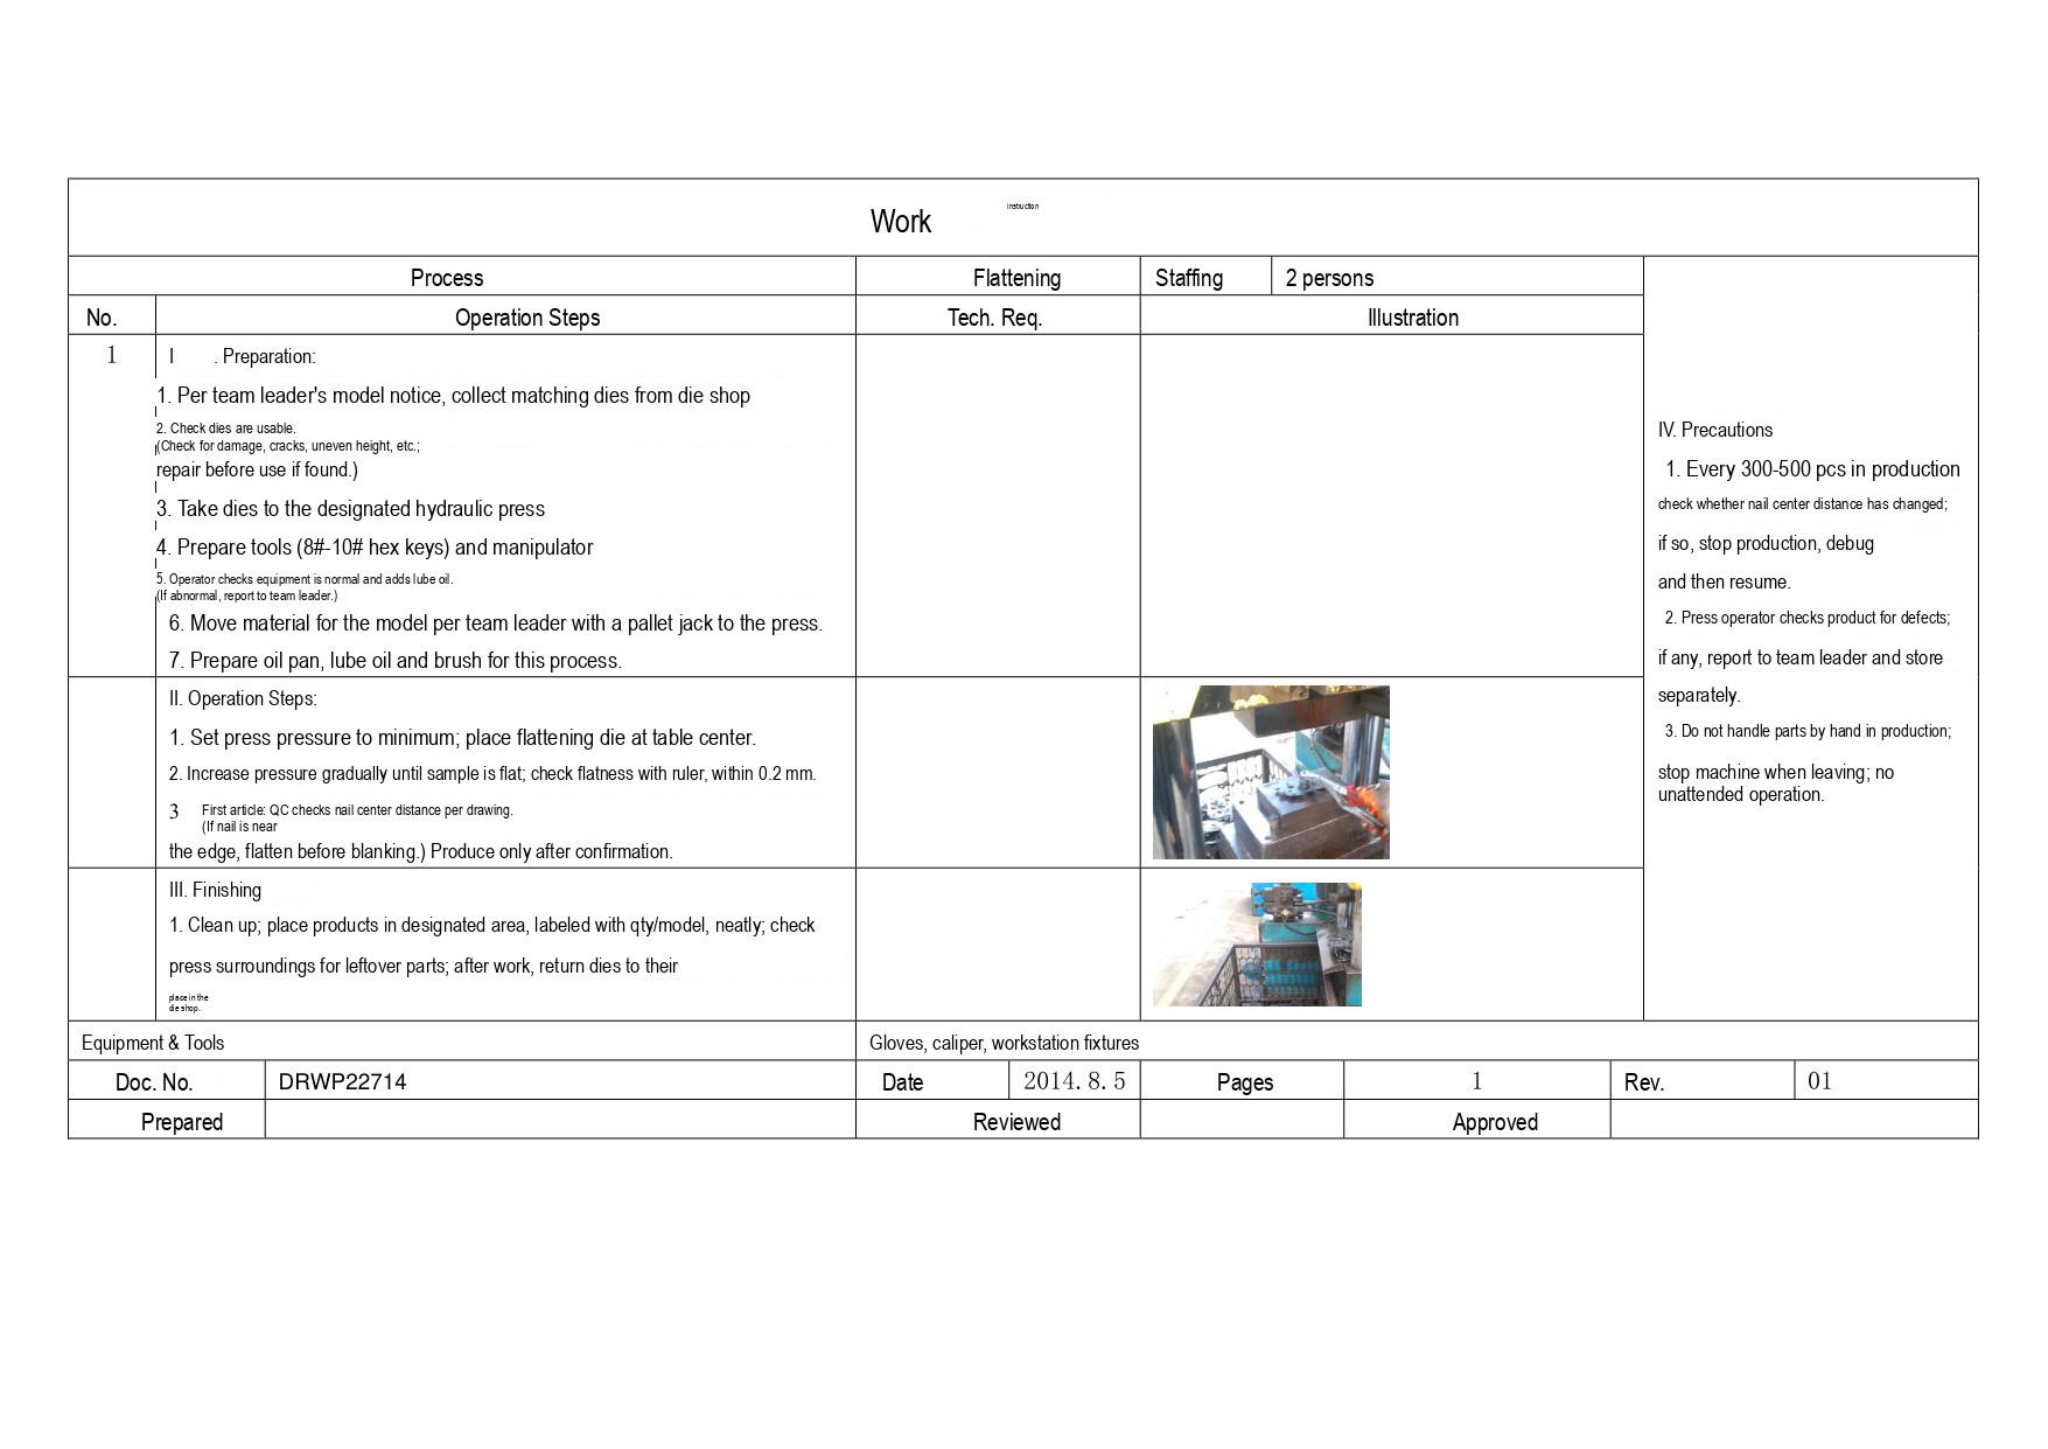Work Instruction

| Process | | Flattening | Staffing | 2 persons |
|---|---|---|---|---|
| **No.** | **Operation Steps** | **Tech. Req.** | **Illustration** | |
| 1 | I. Preparation:<br>1. Per team leader's model notice, collect matching dies from die shop<br>2. Check dies are usable. (Check for damage, cracks, uneven height, etc.; repair before use if found.)<br>3. Take dies to the designated hydraulic press<br>4. Prepare tools (8#-10# hex keys) and manipulator<br>5. Operator checks equipment is normal and adds lube oil. (If abnormal, report to team leader.)<br>6. Move material for the model per team leader with a pallet jack to the press.<br>7. Prepare oil pan, lube oil and brush for this process. | | | |
| | II. Operation Steps:<br>1. Set press pressure to minimum; place flattening die at table center.<br>2. Increase pressure gradually until sample is flat; check flatness with ruler, within 0.2 mm.<br>3 First article: QC checks nail center distance per drawing. (If nail is near the edge, flatten before blanking.) Produce only after confirmation. | | | |
| | III. Finishing<br>1. Clean up; place products in designated area, labeled with qty/model, neatly; check press surroundings for leftover parts; after work, return dies to their place in the die shop. | | | |

IV. Precautions
1. Every 300-500 pcs in production check whether nail center distance has changed; if so, stop production, debug and then resume.
2. Press operator checks product for defects; if any, report to team leader and store separately.
3. Do not handle parts by hand in production; stop machine when leaving; no unattended operation.

| Equipment & Tools | Gloves, caliper, workstation fixtures |
|---|---|

| Doc. No. | DRWP22714 | Date | 2014. 8. 5 | Pages | 1 | Rev. | 01 |
|---|---|---|---|---|---|---|---|
| Prepared | | Reviewed | | Approved | | | |